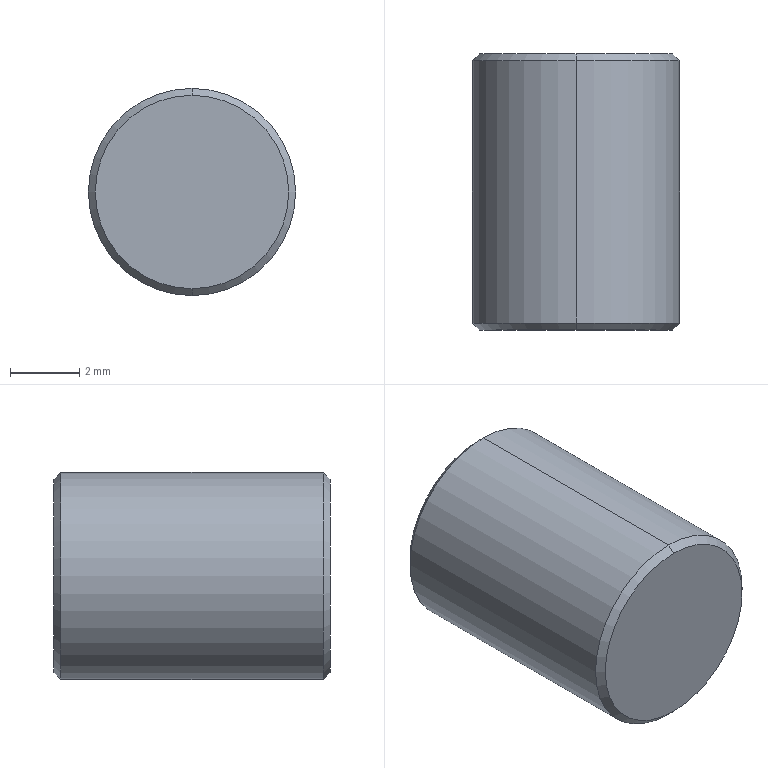Part | SolidWorks | features Chamfer 1, Extrusion 1 | 1 solid | 8 faces | box 6 x 8 x 6 mm | volume 225.457 mm3 | cone 4 | cylinder 2 | plane 2 | commonest cylinder face diameters 6 x2
STEP:
#1=CARTESIAN_POINT('',(0.,8.,2.8));
#2=VERTEX_POINT('',#1);
#3=CARTESIAN_POINT('',(0.,8.,-2.8));
#4=VERTEX_POINT('',#3);
#5=CARTESIAN_POINT('',(0.,8.,0.));
#6=DIRECTION('',(0.,1.,0.));
#7=DIRECTION('',(0.,0.,1.));
#8=AXIS2_PLACEMENT_3D('',#5,#6,#7);
#9=CIRCLE('',#8,2.8);
#10=EDGE_CURVE('',#2,#4,#9,.T.);
#11=ORIENTED_EDGE('',*,*,#10,.F.);
#12=CARTESIAN_POINT('',(0.,7.8,3.));
#13=VERTEX_POINT('',#12);
#14=CARTESIAN_POINT('',(0.,8.,2.8));
#15=DIRECTION('',(0.,-0.7071,0.7071));
#16=VECTOR('',#15,1000.);
#17=LINE('',#14,#16);
#18=EDGE_CURVE('',#2,#13,#17,.T.);
#19=ORIENTED_EDGE('',*,*,#18,.T.);
#20=CARTESIAN_POINT('',(0.,7.8,-3.));
#21=VERTEX_POINT('',#20);
#22=CARTESIAN_POINT('',(0.,7.8,0.));
#23=DIRECTION('',(0.,-1.,0.));
#24=DIRECTION('',(0.,0.,1.));
#25=AXIS2_PLACEMENT_3D('',#22,#23,#24);
#26=CIRCLE('',#25,3.);
#27=EDGE_CURVE('',#21,#13,#26,.T.);
#28=ORIENTED_EDGE('',*,*,#27,.F.);
#29=CARTESIAN_POINT('',(0.,8.,-2.8));
#30=DIRECTION('',(0.,-0.7071,-0.7071));
#31=VECTOR('',#30,1000.);
#32=LINE('',#29,#31);
#33=EDGE_CURVE('',#4,#21,#32,.T.);
#34=ORIENTED_EDGE('',*,*,#33,.F.);
#35=EDGE_LOOP('',(#11,#19,#28,#34));
#36=FACE_OUTER_BOUND('',#35,.T.);
#37=CARTESIAN_POINT('',(0.,8.,0.));
#38=DIRECTION('',(0.,-1.,0.));
#39=DIRECTION('',(0.,0.,-1.));
#40=AXIS2_PLACEMENT_3D('',#37,#38,#39);
#41=CONICAL_SURFACE('',#40,2.8,0.7854);
#42=ADVANCED_FACE('',(#36),#41,.T.);
#43=CARTESIAN_POINT('',(0.,0.,-2.8));
#44=VERTEX_POINT('',#43);
#45=CARTESIAN_POINT('',(0.,0.,2.8));
#46=VERTEX_POINT('',#45);
#47=CARTESIAN_POINT('',(0.,0.,0.));
#48=DIRECTION('',(0.,-1.,0.));
#49=DIRECTION('',(0.,0.,1.));
#50=AXIS2_PLACEMENT_3D('',#47,#48,#49);
#51=CIRCLE('',#50,2.8);
#52=EDGE_CURVE('',#44,#46,#51,.T.);
#53=ORIENTED_EDGE('',*,*,#52,.F.);
#54=CARTESIAN_POINT('',(0.,0.2,-3.));
#55=VERTEX_POINT('',#54);
#56=CARTESIAN_POINT('',(0.,0.2,-3.));
#57=DIRECTION('',(0.,0.7071,-0.7071));
#58=VECTOR('',#57,1000.);
#59=LINE('',#56,#58);
#60=EDGE_CURVE('',#44,#55,#59,.T.);
#61=ORIENTED_EDGE('',*,*,#60,.T.);
#62=CARTESIAN_POINT('',(0.,0.2,3.));
#63=VERTEX_POINT('',#62);
#64=CARTESIAN_POINT('',(0.,0.2,0.));
#65=DIRECTION('',(0.,1.,0.));
#66=DIRECTION('',(0.,0.,1.));
#67=AXIS2_PLACEMENT_3D('',#64,#65,#66);
#68=CIRCLE('',#67,3.);
#69=EDGE_CURVE('',#63,#55,#68,.T.);
#70=ORIENTED_EDGE('',*,*,#69,.F.);
#71=CARTESIAN_POINT('',(0.,0.2,3.));
#72=DIRECTION('',(0.,0.7071,0.7071));
#73=VECTOR('',#72,1000.);
#74=LINE('',#71,#73);
#75=EDGE_CURVE('',#46,#63,#74,.T.);
#76=ORIENTED_EDGE('',*,*,#75,.F.);
#77=EDGE_LOOP('',(#53,#61,#70,#76));
#78=FACE_OUTER_BOUND('',#77,.T.);
#79=CARTESIAN_POINT('',(0.,0.2,0.));
#80=DIRECTION('',(0.,1.,0.));
#81=DIRECTION('',(0.,0.,1.));
#82=AXIS2_PLACEMENT_3D('',#79,#80,#81);
#83=CONICAL_SURFACE('',#82,3.,0.7854);
#84=ADVANCED_FACE('',(#78),#83,.T.);
#85=ORIENTED_EDGE('',*,*,#27,.T.);
#86=CARTESIAN_POINT('',(0.,8.,3.));
#87=DIRECTION('',(0.,-1.,0.));
#88=VECTOR('',#87,1000.);
#89=LINE('',#86,#88);
#90=EDGE_CURVE('',#13,#63,#89,.T.);
#91=ORIENTED_EDGE('',*,*,#90,.T.);
#92=ORIENTED_EDGE('',*,*,#69,.T.);
#93=CARTESIAN_POINT('',(0.,8.,-3.));
#94=DIRECTION('',(0.,-1.,0.));
#95=VECTOR('',#94,1000.);
#96=LINE('',#93,#95);
#97=EDGE_CURVE('',#21,#55,#96,.T.);
#98=ORIENTED_EDGE('',*,*,#97,.F.);
#99=EDGE_LOOP('',(#85,#91,#92,#98));
#100=FACE_OUTER_BOUND('',#99,.T.);
#101=CARTESIAN_POINT('',(0.,8.,0.));
#102=DIRECTION('',(0.,-1.,0.));
#103=DIRECTION('',(0.,0.,-1.));
#104=AXIS2_PLACEMENT_3D('',#101,#102,#103);
#105=CYLINDRICAL_SURFACE('',#104,3.);
#106=ADVANCED_FACE('',(#100),#105,.T.);
#107=ORIENTED_EDGE('',*,*,#90,.F.);
#108=CARTESIAN_POINT('',(0.,7.8,0.));
#109=DIRECTION('',(0.,-1.,0.));
#110=DIRECTION('',(0.,0.,1.));
#111=AXIS2_PLACEMENT_3D('',#108,#109,#110);
#112=CIRCLE('',#111,3.);
#113=EDGE_CURVE('',#13,#21,#112,.T.);
#114=ORIENTED_EDGE('',*,*,#113,.T.);
#115=ORIENTED_EDGE('',*,*,#97,.T.);
#116=CARTESIAN_POINT('',(0.,0.2,0.));
#117=DIRECTION('',(0.,1.,0.));
#118=DIRECTION('',(0.,0.,1.));
#119=AXIS2_PLACEMENT_3D('',#116,#117,#118);
#120=CIRCLE('',#119,3.);
#121=EDGE_CURVE('',#55,#63,#120,.T.);
#122=ORIENTED_EDGE('',*,*,#121,.T.);
#123=EDGE_LOOP('',(#107,#114,#115,#122));
#124=FACE_OUTER_BOUND('',#123,.T.);
#125=CARTESIAN_POINT('',(0.,8.,0.));
#126=DIRECTION('',(0.,-1.,0.));
#127=DIRECTION('',(0.,0.,-1.));
#128=AXIS2_PLACEMENT_3D('',#125,#126,#127);
#129=CYLINDRICAL_SURFACE('',#128,3.);
#130=ADVANCED_FACE('',(#124),#129,.T.);
#131=CARTESIAN_POINT('',(0.,8.,0.));
#132=DIRECTION('',(0.,1.,0.));
#133=DIRECTION('',(0.,0.,1.));
#134=AXIS2_PLACEMENT_3D('',#131,#132,#133);
#135=CIRCLE('',#134,2.8);
#136=EDGE_CURVE('',#4,#2,#135,.T.);
#137=ORIENTED_EDGE('',*,*,#136,.T.);
#138=ORIENTED_EDGE('',*,*,#10,.T.);
#139=EDGE_LOOP('',(#137,#138));
#140=FACE_OUTER_BOUND('',#139,.T.);
#141=CARTESIAN_POINT('',(0.,8.,0.));
#142=DIRECTION('',(0.,1.,0.));
#143=DIRECTION('',(0.,0.,1.));
#144=AXIS2_PLACEMENT_3D('',#141,#142,#143);
#145=PLANE('',#144);
#146=ADVANCED_FACE('',(#140),#145,.T.);
#147=CARTESIAN_POINT('',(0.,0.,0.));
#148=DIRECTION('',(0.,-1.,0.));
#149=DIRECTION('',(0.,0.,1.));
#150=AXIS2_PLACEMENT_3D('',#147,#148,#149);
#151=CIRCLE('',#150,2.8);
#152=EDGE_CURVE('',#46,#44,#151,.T.);
#153=ORIENTED_EDGE('',*,*,#152,.T.);
#154=ORIENTED_EDGE('',*,*,#52,.T.);
#155=EDGE_LOOP('',(#153,#154));
#156=FACE_OUTER_BOUND('',#155,.T.);
#157=CARTESIAN_POINT('',(0.,0.,0.));
#158=DIRECTION('',(0.,1.,0.));
#159=DIRECTION('',(0.,0.,1.));
#160=AXIS2_PLACEMENT_3D('',#157,#158,#159);
#161=PLANE('',#160);
#162=ADVANCED_FACE('',(#156),#161,.F.);
#163=ORIENTED_EDGE('',*,*,#60,.F.);
#164=ORIENTED_EDGE('',*,*,#152,.F.);
#165=ORIENTED_EDGE('',*,*,#75,.T.);
#166=ORIENTED_EDGE('',*,*,#121,.F.);
#167=EDGE_LOOP('',(#163,#164,#165,#166));
#168=FACE_OUTER_BOUND('',#167,.T.);
#169=CARTESIAN_POINT('',(0.,0.2,0.));
#170=DIRECTION('',(0.,1.,0.));
#171=DIRECTION('',(0.,0.,1.));
#172=AXIS2_PLACEMENT_3D('',#169,#170,#171);
#173=CONICAL_SURFACE('',#172,3.,0.7854);
#174=ADVANCED_FACE('',(#168),#173,.T.);
#175=ORIENTED_EDGE('',*,*,#18,.F.);
#176=ORIENTED_EDGE('',*,*,#136,.F.);
#177=ORIENTED_EDGE('',*,*,#33,.T.);
#178=ORIENTED_EDGE('',*,*,#113,.F.);
#179=EDGE_LOOP('',(#175,#176,#177,#178));
#180=FACE_OUTER_BOUND('',#179,.T.);
#181=CARTESIAN_POINT('',(0.,8.,0.));
#182=DIRECTION('',(0.,-1.,0.));
#183=DIRECTION('',(0.,0.,-1.));
#184=AXIS2_PLACEMENT_3D('',#181,#182,#183);
#185=CONICAL_SURFACE('',#184,2.8,0.7854);
#186=ADVANCED_FACE('',(#180),#185,.T.);
#187=CLOSED_SHELL('',(#42,#84,#106,#130,#146,#162,#174,#186));
#188=MANIFOLD_SOLID_BREP('',#187);
#189=CARTESIAN_POINT('',(0.,0.,0.));
#190=DIRECTION('',(0.,0.,1.));
#191=DIRECTION('',(1.,0.,0.));
#192=AXIS2_PLACEMENT_3D('',#189,#190,#191);
#193=(LENGTH_UNIT()NAMED_UNIT(*)SI_UNIT(.MILLI.,.METRE.));
#194=UNCERTAINTY_MEASURE_WITH_UNIT(LENGTH_MEASURE(0.00001),#193,'','');
#195=(NAMED_UNIT(*)PLANE_ANGLE_UNIT()SI_UNIT($,.RADIAN.));
#196=(NAMED_UNIT(*)SI_UNIT($,.STERADIAN.)SOLID_ANGLE_UNIT());
#197=(GEOMETRIC_REPRESENTATION_CONTEXT(3)GLOBAL_UNCERTAINTY_ASSIGNED_CONTEXT((#194))GLOBAL_UNIT_ASSIGNED_CONTEXT((#193,#195,#196))REPRESENTATION_CONTEXT('',''));
#198=ADVANCED_BREP_SHAPE_REPRESENTATION('',(#188,#192),#197);